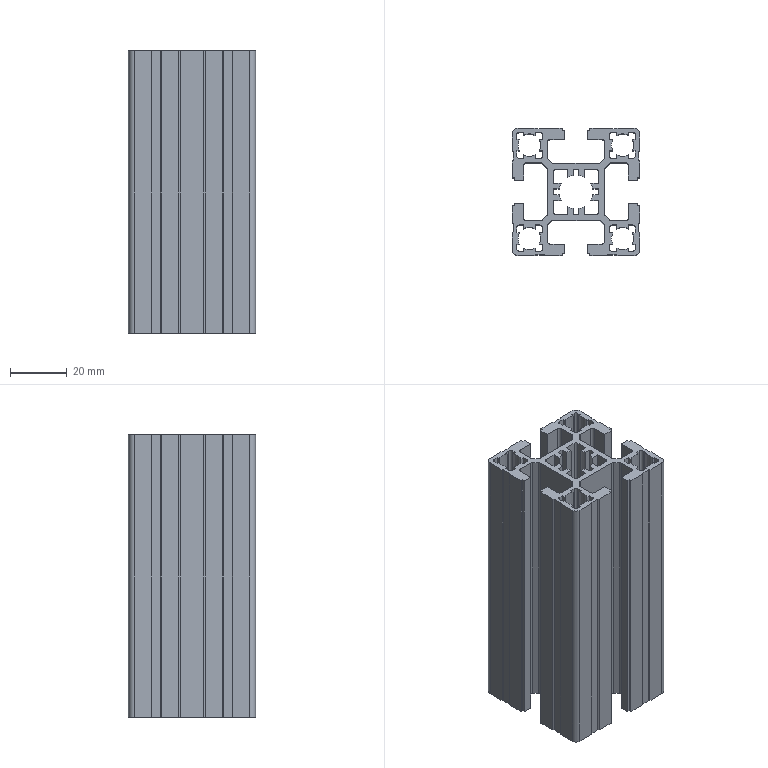Part | STEP file | 4545-100 Al (rack asm 3) | 1 solid | 262 faces | box 45 x 45 x 100 mm | volume 69385 mm3 | plane 186 | cylinder 76 | commonest cylinder face diameters 2 x44 8 x20 12 x8 4 x4